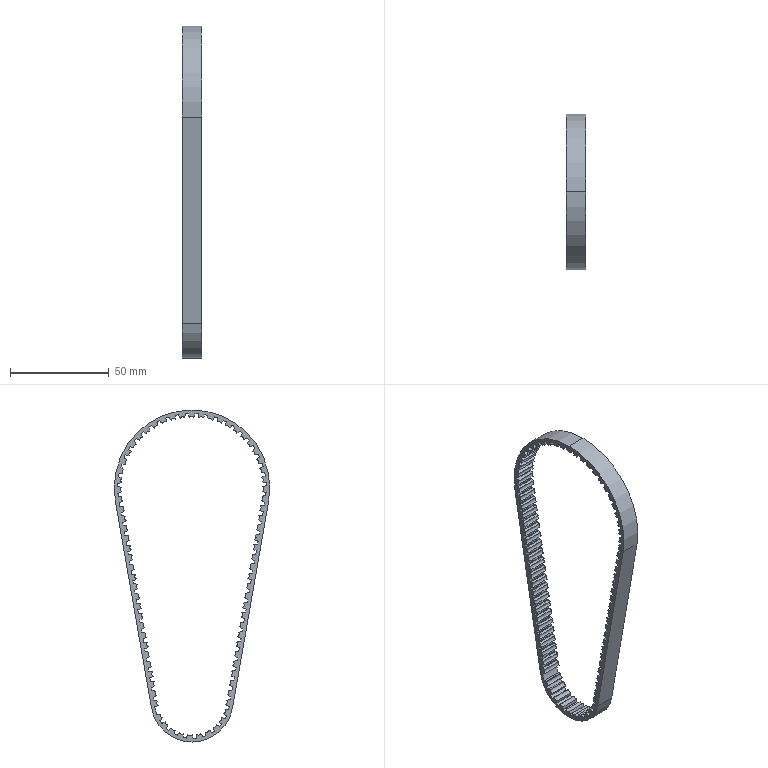Part | SolidWorks | features CurvePattern 1, ExtruThin 1, ICE 1 | 1 solid | 555 faces | box 10 x 78.83 x 168.305 mm | volume 10817 mm3 | cylinder 508 | plane 47 | commonest cylinder face diameters 6.5 x205 0.4 x172 3.003 x91 75.25 x26 38.2 x11 78.83 x2